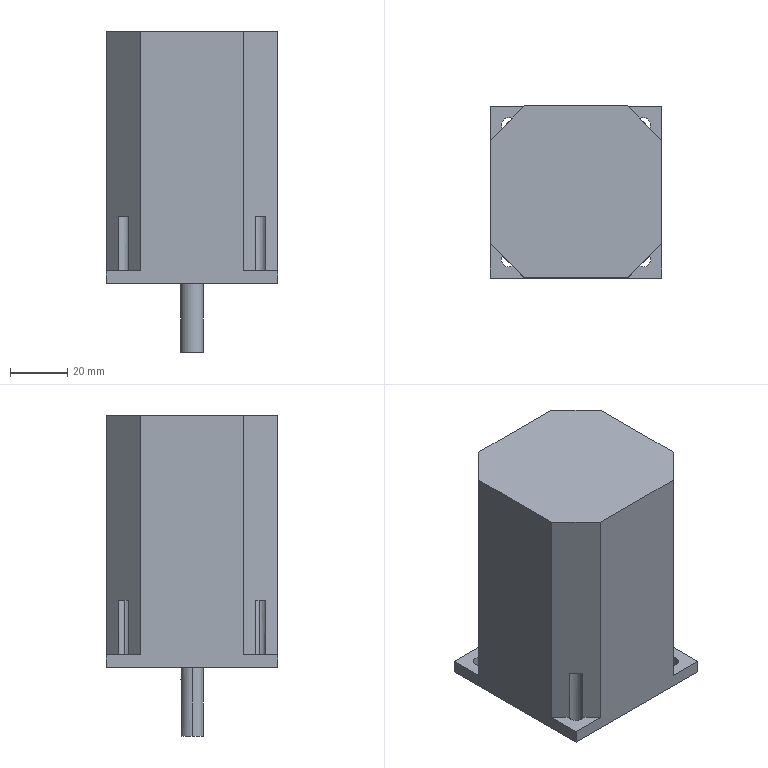Part | 1 solid | 31 faces | box 60 x 60 x 112 mm | volume 292604 mm3 | plane 21 | cylinder 10 | commonest cylinder face diameters 5 x8 8 x2
STEP:
#1=CARTESIAN_POINT('',(-4.,0.,-24.));
#2=VERTEX_POINT('',#1);
#3=CARTESIAN_POINT('',(-1.936,3.5,-24.));
#4=VERTEX_POINT('',#3);
#5=CARTESIAN_POINT('',(0.,0.,-24.));
#6=DIRECTION('',(0.,0.,-1.));
#7=DIRECTION('',(-1.,0.,0.));
#8=AXIS2_PLACEMENT_3D('',#5,#6,#7);
#9=CIRCLE('',#8,4.);
#10=EDGE_CURVE('',#2,#4,#9,.T.);
#11=ORIENTED_EDGE('',*,*,#10,.F.);
#12=CARTESIAN_POINT('',(-4.,0.,0.));
#13=VERTEX_POINT('',#12);
#14=CARTESIAN_POINT('',(-4.,0.,-24.));
#15=DIRECTION('',(0.,0.,1.));
#16=VECTOR('',#15,1000.);
#17=LINE('',#14,#16);
#18=EDGE_CURVE('',#2,#13,#17,.T.);
#19=ORIENTED_EDGE('',*,*,#18,.T.);
#20=CARTESIAN_POINT('',(4.,0.,0.));
#21=VERTEX_POINT('',#20);
#22=CARTESIAN_POINT('',(0.,0.,0.));
#23=DIRECTION('',(0.,0.,-1.));
#24=DIRECTION('',(-1.,0.,0.));
#25=AXIS2_PLACEMENT_3D('',#22,#23,#24);
#26=CIRCLE('',#25,4.);
#27=EDGE_CURVE('',#13,#21,#26,.T.);
#28=ORIENTED_EDGE('',*,*,#27,.T.);
#29=CARTESIAN_POINT('',(4.,0.,-24.));
#30=VERTEX_POINT('',#29);
#31=CARTESIAN_POINT('',(4.,0.,-24.));
#32=DIRECTION('',(0.,0.,1.));
#33=VECTOR('',#32,1000.);
#34=LINE('',#31,#33);
#35=EDGE_CURVE('',#30,#21,#34,.T.);
#36=ORIENTED_EDGE('',*,*,#35,.F.);
#37=CARTESIAN_POINT('',(1.936,3.5,-24.));
#38=VERTEX_POINT('',#37);
#39=CARTESIAN_POINT('',(0.,0.,-24.));
#40=DIRECTION('',(0.,0.,-1.));
#41=DIRECTION('',(-1.,0.,0.));
#42=AXIS2_PLACEMENT_3D('',#39,#40,#41);
#43=CIRCLE('',#42,4.);
#44=EDGE_CURVE('',#38,#30,#43,.T.);
#45=ORIENTED_EDGE('',*,*,#44,.F.);
#46=CARTESIAN_POINT('',(1.936,3.5,-4.));
#47=VERTEX_POINT('',#46);
#48=CARTESIAN_POINT('',(1.936,3.5,-24.));
#49=DIRECTION('',(0.,0.,1.));
#50=VECTOR('',#49,1000.);
#51=LINE('',#48,#50);
#52=EDGE_CURVE('',#38,#47,#51,.T.);
#53=ORIENTED_EDGE('',*,*,#52,.T.);
#54=CARTESIAN_POINT('',(-1.936,3.5,-4.));
#55=VERTEX_POINT('',#54);
#56=CARTESIAN_POINT('',(0.,0.,-4.));
#57=DIRECTION('',(0.,0.,1.));
#58=DIRECTION('',(1.,0.,0.));
#59=AXIS2_PLACEMENT_3D('',#56,#57,#58);
#60=CIRCLE('',#59,4.);
#61=EDGE_CURVE('',#47,#55,#60,.T.);
#62=ORIENTED_EDGE('',*,*,#61,.T.);
#63=CARTESIAN_POINT('',(-1.936,3.5,-24.));
#64=DIRECTION('',(0.,0.,-1.));
#65=VECTOR('',#64,1000.);
#66=LINE('',#63,#65);
#67=EDGE_CURVE('',#55,#4,#66,.T.);
#68=ORIENTED_EDGE('',*,*,#67,.T.);
#69=EDGE_LOOP('',(#11,#19,#28,#36,#45,#53,#62,#68));
#70=FACE_OUTER_BOUND('',#69,.T.);
#71=CARTESIAN_POINT('',(0.,0.,-24.));
#72=DIRECTION('',(0.,0.,1.));
#73=DIRECTION('',(1.,0.,0.));
#74=AXIS2_PLACEMENT_3D('',#71,#72,#73);
#75=CYLINDRICAL_SURFACE('',#74,4.);
#76=ADVANCED_FACE('',(#70),#75,.T.);
#77=CARTESIAN_POINT('',(-21.07,-23.57,23.5));
#78=VERTEX_POINT('',#77);
#79=CARTESIAN_POINT('',(-22.285,-25.715,23.5));
#80=VERTEX_POINT('',#79);
#81=CARTESIAN_POINT('',(-23.57,-23.57,23.5));
#82=DIRECTION('',(0.,0.,-1.));
#83=DIRECTION('',(-1.,0.,0.));
#84=AXIS2_PLACEMENT_3D('',#81,#82,#83);
#85=CIRCLE('',#84,2.5);
#86=EDGE_CURVE('',#78,#80,#85,.T.);
#87=ORIENTED_EDGE('',*,*,#86,.F.);
#88=CARTESIAN_POINT('',(-21.07,-23.57,0.));
#89=VERTEX_POINT('',#88);
#90=CARTESIAN_POINT('',(-21.07,-23.57,23.5));
#91=DIRECTION('',(0.,0.,-1.));
#92=VECTOR('',#91,1000.);
#93=LINE('',#90,#92);
#94=EDGE_CURVE('',#78,#89,#93,.T.);
#95=ORIENTED_EDGE('',*,*,#94,.T.);
#96=CARTESIAN_POINT('',(-26.07,-23.57,0.));
#97=VERTEX_POINT('',#96);
#98=CARTESIAN_POINT('',(-23.57,-23.57,0.));
#99=DIRECTION('',(0.,0.,-1.));
#100=DIRECTION('',(-1.,0.,0.));
#101=AXIS2_PLACEMENT_3D('',#98,#99,#100);
#102=CIRCLE('',#101,2.5);
#103=EDGE_CURVE('',#89,#97,#102,.T.);
#104=ORIENTED_EDGE('',*,*,#103,.T.);
#105=CARTESIAN_POINT('',(-26.07,-23.57,4.5));
#106=VERTEX_POINT('',#105);
#107=CARTESIAN_POINT('',(-26.07,-23.57,23.5));
#108=DIRECTION('',(0.,0.,-1.));
#109=VECTOR('',#108,1000.);
#110=LINE('',#107,#109);
#111=EDGE_CURVE('',#106,#97,#110,.T.);
#112=ORIENTED_EDGE('',*,*,#111,.F.);
#113=CARTESIAN_POINT('',(-22.285,-25.715,4.5));
#114=VERTEX_POINT('',#113);
#115=CARTESIAN_POINT('',(-23.57,-23.57,4.5));
#116=DIRECTION('',(0.,0.,-1.));
#117=DIRECTION('',(-1.,0.,0.));
#118=AXIS2_PLACEMENT_3D('',#115,#116,#117);
#119=CIRCLE('',#118,2.5);
#120=EDGE_CURVE('',#114,#106,#119,.T.);
#121=ORIENTED_EDGE('',*,*,#120,.F.);
#122=CARTESIAN_POINT('',(-22.285,-25.715,23.5));
#123=DIRECTION('',(0.,0.,-1.));
#124=VECTOR('',#123,1000.);
#125=LINE('',#122,#124);
#126=EDGE_CURVE('',#80,#114,#125,.T.);
#127=ORIENTED_EDGE('',*,*,#126,.F.);
#128=EDGE_LOOP('',(#87,#95,#104,#112,#121,#127));
#129=FACE_OUTER_BOUND('',#128,.T.);
#130=CARTESIAN_POINT('',(-23.57,-23.57,23.5));
#131=DIRECTION('',(0.,0.,-1.));
#132=DIRECTION('',(-1.,0.,0.));
#133=AXIS2_PLACEMENT_3D('',#130,#131,#132);
#134=CYLINDRICAL_SURFACE('',#133,2.5);
#135=ADVANCED_FACE('',(#129),#134,.F.);
#136=CARTESIAN_POINT('',(22.285,-25.715,4.5));
#137=VERTEX_POINT('',#136);
#138=CARTESIAN_POINT('',(26.07,-23.57,4.5));
#139=VERTEX_POINT('',#138);
#140=CARTESIAN_POINT('',(23.57,-23.57,4.5));
#141=DIRECTION('',(0.,0.,1.));
#142=DIRECTION('',(1.,0.,0.));
#143=AXIS2_PLACEMENT_3D('',#140,#141,#142);
#144=CIRCLE('',#143,2.5);
#145=EDGE_CURVE('',#137,#139,#144,.T.);
#146=ORIENTED_EDGE('',*,*,#145,.T.);
#147=CARTESIAN_POINT('',(26.07,-23.57,0.));
#148=VERTEX_POINT('',#147);
#149=CARTESIAN_POINT('',(26.07,-23.57,23.5));
#150=DIRECTION('',(0.,0.,-1.));
#151=VECTOR('',#150,1000.);
#152=LINE('',#149,#151);
#153=EDGE_CURVE('',#139,#148,#152,.T.);
#154=ORIENTED_EDGE('',*,*,#153,.T.);
#155=CARTESIAN_POINT('',(21.07,-23.57,0.));
#156=VERTEX_POINT('',#155);
#157=CARTESIAN_POINT('',(23.57,-23.57,0.));
#158=DIRECTION('',(0.,0.,-1.));
#159=DIRECTION('',(-1.,0.,0.));
#160=AXIS2_PLACEMENT_3D('',#157,#158,#159);
#161=CIRCLE('',#160,2.5);
#162=EDGE_CURVE('',#148,#156,#161,.T.);
#163=ORIENTED_EDGE('',*,*,#162,.T.);
#164=CARTESIAN_POINT('',(21.07,-23.57,23.5));
#165=VERTEX_POINT('',#164);
#166=CARTESIAN_POINT('',(21.07,-23.57,23.5));
#167=DIRECTION('',(0.,0.,-1.));
#168=VECTOR('',#167,1000.);
#169=LINE('',#166,#168);
#170=EDGE_CURVE('',#165,#156,#169,.T.);
#171=ORIENTED_EDGE('',*,*,#170,.F.);
#172=CARTESIAN_POINT('',(22.285,-25.715,23.5));
#173=VERTEX_POINT('',#172);
#174=CARTESIAN_POINT('',(23.57,-23.57,23.5));
#175=DIRECTION('',(0.,0.,-1.));
#176=DIRECTION('',(-1.,0.,0.));
#177=AXIS2_PLACEMENT_3D('',#174,#175,#176);
#178=CIRCLE('',#177,2.5);
#179=EDGE_CURVE('',#173,#165,#178,.T.);
#180=ORIENTED_EDGE('',*,*,#179,.F.);
#181=CARTESIAN_POINT('',(22.285,-25.715,23.5));
#182=DIRECTION('',(0.,0.,1.));
#183=VECTOR('',#182,1000.);
#184=LINE('',#181,#183);
#185=EDGE_CURVE('',#137,#173,#184,.T.);
#186=ORIENTED_EDGE('',*,*,#185,.F.);
#187=EDGE_LOOP('',(#146,#154,#163,#171,#180,#186));
#188=FACE_OUTER_BOUND('',#187,.T.);
#189=CARTESIAN_POINT('',(23.57,-23.57,23.5));
#190=DIRECTION('',(0.,0.,-1.));
#191=DIRECTION('',(-1.,0.,0.));
#192=AXIS2_PLACEMENT_3D('',#189,#190,#191);
#193=CYLINDRICAL_SURFACE('',#192,2.5);
#194=ADVANCED_FACE('',(#188),#193,.F.);
#195=CARTESIAN_POINT('',(-21.07,23.57,23.5));
#196=VERTEX_POINT('',#195);
#197=CARTESIAN_POINT('',(-25.715,22.285,23.5));
#198=VERTEX_POINT('',#197);
#199=CARTESIAN_POINT('',(-23.57,23.57,23.5));
#200=DIRECTION('',(0.,0.,-1.));
#201=DIRECTION('',(-1.,0.,0.));
#202=AXIS2_PLACEMENT_3D('',#199,#200,#201);
#203=CIRCLE('',#202,2.5);
#204=EDGE_CURVE('',#196,#198,#203,.T.);
#205=ORIENTED_EDGE('',*,*,#204,.F.);
#206=CARTESIAN_POINT('',(-21.07,23.57,0.));
#207=VERTEX_POINT('',#206);
#208=CARTESIAN_POINT('',(-21.07,23.57,23.5));
#209=DIRECTION('',(0.,0.,-1.));
#210=VECTOR('',#209,1000.);
#211=LINE('',#208,#210);
#212=EDGE_CURVE('',#196,#207,#211,.T.);
#213=ORIENTED_EDGE('',*,*,#212,.T.);
#214=CARTESIAN_POINT('',(-26.07,23.57,0.));
#215=VERTEX_POINT('',#214);
#216=CARTESIAN_POINT('',(-23.57,23.57,0.));
#217=DIRECTION('',(0.,0.,-1.));
#218=DIRECTION('',(-1.,0.,0.));
#219=AXIS2_PLACEMENT_3D('',#216,#217,#218);
#220=CIRCLE('',#219,2.5);
#221=EDGE_CURVE('',#207,#215,#220,.T.);
#222=ORIENTED_EDGE('',*,*,#221,.T.);
#223=CARTESIAN_POINT('',(-26.07,23.57,4.5));
#224=VERTEX_POINT('',#223);
#225=CARTESIAN_POINT('',(-26.07,23.57,23.5));
#226=DIRECTION('',(0.,0.,-1.));
#227=VECTOR('',#226,1000.);
#228=LINE('',#225,#227);
#229=EDGE_CURVE('',#224,#215,#228,.T.);
#230=ORIENTED_EDGE('',*,*,#229,.F.);
#231=CARTESIAN_POINT('',(-25.715,22.285,4.5));
#232=VERTEX_POINT('',#231);
#233=CARTESIAN_POINT('',(-23.57,23.57,4.5));
#234=DIRECTION('',(0.,0.,1.));
#235=DIRECTION('',(1.,0.,0.));
#236=AXIS2_PLACEMENT_3D('',#233,#234,#235);
#237=CIRCLE('',#236,2.5);
#238=EDGE_CURVE('',#224,#232,#237,.T.);
#239=ORIENTED_EDGE('',*,*,#238,.T.);
#240=CARTESIAN_POINT('',(-25.715,22.285,23.5));
#241=DIRECTION('',(0.,0.,-1.));
#242=VECTOR('',#241,1000.);
#243=LINE('',#240,#242);
#244=EDGE_CURVE('',#198,#232,#243,.T.);
#245=ORIENTED_EDGE('',*,*,#244,.F.);
#246=EDGE_LOOP('',(#205,#213,#222,#230,#239,#245));
#247=FACE_OUTER_BOUND('',#246,.T.);
#248=CARTESIAN_POINT('',(-23.57,23.57,23.5));
#249=DIRECTION('',(0.,0.,-1.));
#250=DIRECTION('',(-1.,0.,0.));
#251=AXIS2_PLACEMENT_3D('',#248,#249,#250);
#252=CYLINDRICAL_SURFACE('',#251,2.5);
#253=ADVANCED_FACE('',(#247),#252,.F.);
#254=CARTESIAN_POINT('',(26.07,23.57,4.5));
#255=VERTEX_POINT('',#254);
#256=CARTESIAN_POINT('',(25.715,22.285,4.5));
#257=VERTEX_POINT('',#256);
#258=CARTESIAN_POINT('',(23.57,23.57,4.5));
#259=DIRECTION('',(0.,0.,-1.));
#260=DIRECTION('',(-1.,0.,0.));
#261=AXIS2_PLACEMENT_3D('',#258,#259,#260);
#262=CIRCLE('',#261,2.5);
#263=EDGE_CURVE('',#255,#257,#262,.T.);
#264=ORIENTED_EDGE('',*,*,#263,.F.);
#265=CARTESIAN_POINT('',(26.07,23.57,0.));
#266=VERTEX_POINT('',#265);
#267=CARTESIAN_POINT('',(26.07,23.57,23.5));
#268=DIRECTION('',(0.,0.,-1.));
#269=VECTOR('',#268,1000.);
#270=LINE('',#267,#269);
#271=EDGE_CURVE('',#255,#266,#270,.T.);
#272=ORIENTED_EDGE('',*,*,#271,.T.);
#273=CARTESIAN_POINT('',(21.07,23.57,0.));
#274=VERTEX_POINT('',#273);
#275=CARTESIAN_POINT('',(23.57,23.57,0.));
#276=DIRECTION('',(0.,0.,-1.));
#277=DIRECTION('',(-1.,0.,0.));
#278=AXIS2_PLACEMENT_3D('',#275,#276,#277);
#279=CIRCLE('',#278,2.5);
#280=EDGE_CURVE('',#266,#274,#279,.T.);
#281=ORIENTED_EDGE('',*,*,#280,.T.);
#282=CARTESIAN_POINT('',(21.07,23.57,23.5));
#283=VERTEX_POINT('',#282);
#284=CARTESIAN_POINT('',(21.07,23.57,23.5));
#285=DIRECTION('',(0.,0.,-1.));
#286=VECTOR('',#285,1000.);
#287=LINE('',#284,#286);
#288=EDGE_CURVE('',#283,#274,#287,.T.);
#289=ORIENTED_EDGE('',*,*,#288,.F.);
#290=CARTESIAN_POINT('',(25.715,22.285,23.5));
#291=VERTEX_POINT('',#290);
#292=CARTESIAN_POINT('',(23.57,23.57,23.5));
#293=DIRECTION('',(0.,0.,-1.));
#294=DIRECTION('',(-1.,0.,0.));
#295=AXIS2_PLACEMENT_3D('',#292,#293,#294);
#296=CIRCLE('',#295,2.5);
#297=EDGE_CURVE('',#291,#283,#296,.T.);
#298=ORIENTED_EDGE('',*,*,#297,.F.);
#299=CARTESIAN_POINT('',(25.715,22.285,23.5));
#300=DIRECTION('',(0.,0.,1.));
#301=VECTOR('',#300,1000.);
#302=LINE('',#299,#301);
#303=EDGE_CURVE('',#257,#291,#302,.T.);
#304=ORIENTED_EDGE('',*,*,#303,.F.);
#305=EDGE_LOOP('',(#264,#272,#281,#289,#298,#304));
#306=FACE_OUTER_BOUND('',#305,.T.);
#307=CARTESIAN_POINT('',(23.57,23.57,23.5));
#308=DIRECTION('',(0.,0.,-1.));
#309=DIRECTION('',(-1.,0.,0.));
#310=AXIS2_PLACEMENT_3D('',#307,#308,#309);
#311=CYLINDRICAL_SURFACE('',#310,2.5);
#312=ADVANCED_FACE('',(#306),#311,.F.);
#313=CARTESIAN_POINT('',(30.,-30.,0.));
#314=VERTEX_POINT('',#313);
#315=CARTESIAN_POINT('',(30.,30.,0.));
#316=VERTEX_POINT('',#315);
#317=CARTESIAN_POINT('',(30.,-30.,0.));
#318=DIRECTION('',(0.,1.,0.));
#319=VECTOR('',#318,1000.);
#320=LINE('',#317,#319);
#321=EDGE_CURVE('',#314,#316,#320,.T.);
#322=ORIENTED_EDGE('',*,*,#321,.F.);
#323=CARTESIAN_POINT('',(-30.,-30.,0.));
#324=VERTEX_POINT('',#323);
#325=CARTESIAN_POINT('',(-30.,-30.,0.));
#326=DIRECTION('',(1.,0.,0.));
#327=VECTOR('',#326,1000.);
#328=LINE('',#325,#327);
#329=EDGE_CURVE('',#324,#314,#328,.T.);
#330=ORIENTED_EDGE('',*,*,#329,.F.);
#331=CARTESIAN_POINT('',(-30.,30.,0.));
#332=VERTEX_POINT('',#331);
#333=CARTESIAN_POINT('',(-30.,-30.,0.));
#334=DIRECTION('',(0.,-1.,0.));
#335=VECTOR('',#334,1000.);
#336=LINE('',#333,#335);
#337=EDGE_CURVE('',#332,#324,#336,.T.);
#338=ORIENTED_EDGE('',*,*,#337,.F.);
#339=CARTESIAN_POINT('',(-30.,30.,0.));
#340=DIRECTION('',(-1.,0.,0.));
#341=VECTOR('',#340,1000.);
#342=LINE('',#339,#341);
#343=EDGE_CURVE('',#316,#332,#342,.T.);
#344=ORIENTED_EDGE('',*,*,#343,.F.);
#345=EDGE_LOOP('',(#322,#330,#338,#344));
#346=FACE_OUTER_BOUND('',#345,.T.);
#347=CARTESIAN_POINT('',(23.57,23.57,0.));
#348=DIRECTION('',(0.,0.,-1.));
#349=DIRECTION('',(-1.,0.,0.));
#350=AXIS2_PLACEMENT_3D('',#347,#348,#349);
#351=CIRCLE('',#350,2.5);
#352=EDGE_CURVE('',#274,#266,#351,.T.);
#353=ORIENTED_EDGE('',*,*,#352,.F.);
#354=ORIENTED_EDGE('',*,*,#280,.F.);
#355=EDGE_LOOP('',(#353,#354));
#356=FACE_BOUND('',#355,.T.);
#357=CARTESIAN_POINT('',(-23.57,23.57,0.));
#358=DIRECTION('',(0.,0.,-1.));
#359=DIRECTION('',(-1.,0.,0.));
#360=AXIS2_PLACEMENT_3D('',#357,#358,#359);
#361=CIRCLE('',#360,2.5);
#362=EDGE_CURVE('',#215,#207,#361,.T.);
#363=ORIENTED_EDGE('',*,*,#362,.F.);
#364=ORIENTED_EDGE('',*,*,#221,.F.);
#365=EDGE_LOOP('',(#363,#364));
#366=FACE_BOUND('',#365,.T.);
#367=CARTESIAN_POINT('',(23.57,-23.57,0.));
#368=DIRECTION('',(0.,0.,-1.));
#369=DIRECTION('',(-1.,0.,0.));
#370=AXIS2_PLACEMENT_3D('',#367,#368,#369);
#371=CIRCLE('',#370,2.5);
#372=EDGE_CURVE('',#156,#148,#371,.T.);
#373=ORIENTED_EDGE('',*,*,#372,.F.);
#374=ORIENTED_EDGE('',*,*,#162,.F.);
#375=EDGE_LOOP('',(#373,#374));
#376=FACE_BOUND('',#375,.T.);
#377=CARTESIAN_POINT('',(-23.57,-23.57,0.));
#378=DIRECTION('',(0.,0.,-1.));
#379=DIRECTION('',(-1.,0.,0.));
#380=AXIS2_PLACEMENT_3D('',#377,#378,#379);
#381=CIRCLE('',#380,2.5);
#382=EDGE_CURVE('',#97,#89,#381,.T.);
#383=ORIENTED_EDGE('',*,*,#382,.F.);
#384=ORIENTED_EDGE('',*,*,#103,.F.);
#385=EDGE_LOOP('',(#383,#384));
#386=FACE_BOUND('',#385,.T.);
#387=CARTESIAN_POINT('',(0.,0.,0.));
#388=DIRECTION('',(0.,0.,-1.));
#389=DIRECTION('',(-1.,0.,0.));
#390=AXIS2_PLACEMENT_3D('',#387,#388,#389);
#391=CIRCLE('',#390,4.);
#392=EDGE_CURVE('',#21,#13,#391,.T.);
#393=ORIENTED_EDGE('',*,*,#392,.F.);
#394=ORIENTED_EDGE('',*,*,#27,.F.);
#395=EDGE_LOOP('',(#393,#394));
#396=FACE_BOUND('',#395,.T.);
#397=CARTESIAN_POINT('',(0.,0.,0.));
#398=DIRECTION('',(0.,0.,-1.));
#399=DIRECTION('',(-1.,0.,0.));
#400=AXIS2_PLACEMENT_3D('',#397,#398,#399);
#401=PLANE('',#400);
#402=ADVANCED_FACE('',(#346,#356,#366,#376,#386,#396),#401,.T.);
#403=CARTESIAN_POINT('',(30.,18.,4.5));
#404=VERTEX_POINT('',#403);
#405=CARTESIAN_POINT('',(30.,30.,4.5));
#406=VERTEX_POINT('',#405);
#407=CARTESIAN_POINT('',(30.,30.,4.5));
#408=DIRECTION('',(0.,1.,0.));
#409=VECTOR('',#408,1000.);
#410=LINE('',#407,#409);
#411=EDGE_CURVE('',#404,#406,#410,.T.);
#412=ORIENTED_EDGE('',*,*,#411,.F.);
#413=CARTESIAN_POINT('',(30.,18.,88.));
#414=VERTEX_POINT('',#413);
#415=CARTESIAN_POINT('',(30.,18.,4.5));
#416=DIRECTION('',(0.,0.,1.));
#417=VECTOR('',#416,1000.);
#418=LINE('',#415,#417);
#419=EDGE_CURVE('',#404,#414,#418,.T.);
#420=ORIENTED_EDGE('',*,*,#419,.T.);
#421=CARTESIAN_POINT('',(30.,-18.,88.));
#422=VERTEX_POINT('',#421);
#423=CARTESIAN_POINT('',(30.,-30.,88.));
#424=DIRECTION('',(0.,1.,0.));
#425=VECTOR('',#424,1000.);
#426=LINE('',#423,#425);
#427=EDGE_CURVE('',#422,#414,#426,.T.);
#428=ORIENTED_EDGE('',*,*,#427,.F.);
#429=CARTESIAN_POINT('',(30.,-18.,4.5));
#430=VERTEX_POINT('',#429);
#431=CARTESIAN_POINT('',(30.,-18.,4.5));
#432=DIRECTION('',(0.,0.,1.));
#433=VECTOR('',#432,1000.);
#434=LINE('',#431,#433);
#435=EDGE_CURVE('',#430,#422,#434,.T.);
#436=ORIENTED_EDGE('',*,*,#435,.F.);
#437=CARTESIAN_POINT('',(30.,-30.,4.5));
#438=VERTEX_POINT('',#437);
#439=CARTESIAN_POINT('',(30.,-30.,4.5));
#440=DIRECTION('',(0.,1.,0.));
#441=VECTOR('',#440,1000.);
#442=LINE('',#439,#441);
#443=EDGE_CURVE('',#438,#430,#442,.T.);
#444=ORIENTED_EDGE('',*,*,#443,.F.);
#445=CARTESIAN_POINT('',(30.,-30.,88.));
#446=DIRECTION('',(0.,0.,-1.));
#447=VECTOR('',#446,1000.);
#448=LINE('',#445,#447);
#449=EDGE_CURVE('',#438,#314,#448,.T.);
#450=ORIENTED_EDGE('',*,*,#449,.T.);
#451=ORIENTED_EDGE('',*,*,#321,.T.);
#452=CARTESIAN_POINT('',(30.,30.,88.));
#453=DIRECTION('',(0.,0.,-1.));
#454=VECTOR('',#453,1000.);
#455=LINE('',#452,#454);
#456=EDGE_CURVE('',#406,#316,#455,.T.);
#457=ORIENTED_EDGE('',*,*,#456,.F.);
#458=EDGE_LOOP('',(#412,#420,#428,#436,#444,#450,#451,#457));
#459=FACE_OUTER_BOUND('',#458,.T.);
#460=CARTESIAN_POINT('',(30.,-30.,88.));
#461=DIRECTION('',(-1.,0.,0.));
#462=DIRECTION('',(0.,0.,1.));
#463=AXIS2_PLACEMENT_3D('',#460,#461,#462);
#464=PLANE('',#463);
#465=ADVANCED_FACE('',(#459),#464,.F.);
#466=CARTESIAN_POINT('',(18.,30.,88.));
#467=VERTEX_POINT('',#466);
#468=CARTESIAN_POINT('',(-18.,30.,88.));
#469=VERTEX_POINT('',#468);
#470=CARTESIAN_POINT('',(-30.,30.,88.));
#471=DIRECTION('',(-1.,0.,0.));
#472=VECTOR('',#471,1000.);
#473=LINE('',#470,#472);
#474=EDGE_CURVE('',#467,#469,#473,.T.);
#475=ORIENTED_EDGE('',*,*,#474,.F.);
#476=CARTESIAN_POINT('',(18.,30.,4.5));
#477=VERTEX_POINT('',#476);
#478=CARTESIAN_POINT('',(18.,30.,4.5));
#479=DIRECTION('',(0.,0.,1.));
#480=VECTOR('',#479,1000.);
#481=LINE('',#478,#480);
#482=EDGE_CURVE('',#477,#467,#481,.T.);
#483=ORIENTED_EDGE('',*,*,#482,.F.);
#484=CARTESIAN_POINT('',(18.,30.,4.5));
#485=DIRECTION('',(-1.,0.,0.));
#486=VECTOR('',#485,1000.);
#487=LINE('',#484,#486);
#488=EDGE_CURVE('',#406,#477,#487,.T.);
#489=ORIENTED_EDGE('',*,*,#488,.F.);
#490=ORIENTED_EDGE('',*,*,#456,.T.);
#491=ORIENTED_EDGE('',*,*,#343,.T.);
#492=CARTESIAN_POINT('',(-30.,30.,4.5));
#493=VERTEX_POINT('',#492);
#494=CARTESIAN_POINT('',(-30.,30.,88.));
#495=DIRECTION('',(0.,0.,-1.));
#496=VECTOR('',#495,1000.);
#497=LINE('',#494,#496);
#498=EDGE_CURVE('',#493,#332,#497,.T.);
#499=ORIENTED_EDGE('',*,*,#498,.F.);
#500=CARTESIAN_POINT('',(-18.,30.,4.5));
#501=VERTEX_POINT('',#500);
#502=CARTESIAN_POINT('',(-18.,30.,4.5));
#503=DIRECTION('',(-1.,0.,0.));
#504=VECTOR('',#503,1000.);
#505=LINE('',#502,#504);
#506=EDGE_CURVE('',#501,#493,#505,.T.);
#507=ORIENTED_EDGE('',*,*,#506,.F.);
#508=CARTESIAN_POINT('',(-18.,30.,4.5));
#509=DIRECTION('',(0.,0.,1.));
#510=VECTOR('',#509,1000.);
#511=LINE('',#508,#510);
#512=EDGE_CURVE('',#501,#469,#511,.T.);
#513=ORIENTED_EDGE('',*,*,#512,.T.);
#514=EDGE_LOOP('',(#475,#483,#489,#490,#491,#499,#507,#513));
#515=FACE_OUTER_BOUND('',#514,.T.);
#516=CARTESIAN_POINT('',(-30.,30.,88.));
#517=DIRECTION('',(0.,-1.,0.));
#518=DIRECTION('',(0.,0.,-1.));
#519=AXIS2_PLACEMENT_3D('',#516,#517,#518);
#520=PLANE('',#519);
#521=ADVANCED_FACE('',(#515),#520,.F.);
#522=CARTESIAN_POINT('',(-30.,-18.,4.5));
#523=VERTEX_POINT('',#522);
#524=CARTESIAN_POINT('',(-30.,-30.,4.5));
#525=VERTEX_POINT('',#524);
#526=CARTESIAN_POINT('',(-30.,-30.,4.5));
#527=DIRECTION('',(0.,-1.,0.));
#528=VECTOR('',#527,1000.);
#529=LINE('',#526,#528);
#530=EDGE_CURVE('',#523,#525,#529,.T.);
#531=ORIENTED_EDGE('',*,*,#530,.F.);
#532=CARTESIAN_POINT('',(-30.,-18.,88.));
#533=VERTEX_POINT('',#532);
#534=CARTESIAN_POINT('',(-30.,-18.,4.5));
#535=DIRECTION('',(0.,0.,1.));
#536=VECTOR('',#535,1000.);
#537=LINE('',#534,#536);
#538=EDGE_CURVE('',#523,#533,#537,.T.);
#539=ORIENTED_EDGE('',*,*,#538,.T.);
#540=CARTESIAN_POINT('',(-30.,18.,88.));
#541=VERTEX_POINT('',#540);
#542=CARTESIAN_POINT('',(-30.,-30.,88.));
#543=DIRECTION('',(0.,-1.,0.));
#544=VECTOR('',#543,1000.);
#545=LINE('',#542,#544);
#546=EDGE_CURVE('',#541,#533,#545,.T.);
#547=ORIENTED_EDGE('',*,*,#546,.F.);
#548=CARTESIAN_POINT('',(-30.,18.,4.5));
#549=VERTEX_POINT('',#548);
#550=CARTESIAN_POINT('',(-30.,18.,4.5));
#551=DIRECTION('',(0.,0.,1.));
#552=VECTOR('',#551,1000.);
#553=LINE('',#550,#552);
#554=EDGE_CURVE('',#549,#541,#553,.T.);
#555=ORIENTED_EDGE('',*,*,#554,.F.);
#556=CARTESIAN_POINT('',(-30.,30.,4.5));
#557=DIRECTION('',(0.,-1.,0.));
#558=VECTOR('',#557,1000.);
#559=LINE('',#556,#558);
#560=EDGE_CURVE('',#493,#549,#559,.T.);
#561=ORIENTED_EDGE('',*,*,#560,.F.);
#562=ORIENTED_EDGE('',*,*,#498,.T.);
#563=ORIENTED_EDGE('',*,*,#337,.T.);
#564=CARTESIAN_POINT('',(-30.,-30.,88.));
#565=DIRECTION('',(0.,0.,-1.));
#566=VECTOR('',#565,1000.);
#567=LINE('',#564,#566);
#568=EDGE_CURVE('',#525,#324,#567,.T.);
#569=ORIENTED_EDGE('',*,*,#568,.F.);
#570=EDGE_LOOP('',(#531,#539,#547,#555,#561,#562,#563,#569));
#571=FACE_OUTER_BOUND('',#570,.T.);
#572=CARTESIAN_POINT('',(-30.,-30.,88.));
#573=DIRECTION('',(1.,0.,0.));
#574=DIRECTION('',(0.,0.,-1.));
#575=AXIS2_PLACEMENT_3D('',#572,#573,#574);
#576=PLANE('',#575);
#577=ADVANCED_FACE('',(#571),#576,.F.);
#578=CARTESIAN_POINT('',(18.,-30.,4.5));
#579=VERTEX_POINT('',#578);
#580=CARTESIAN_POINT('',(18.,-30.,4.5));
#581=DIRECTION('',(1.,0.,0.));
#582=VECTOR('',#581,1000.);
#583=LINE('',#580,#582);
#584=EDGE_CURVE('',#579,#438,#583,.T.);
#585=ORIENTED_EDGE('',*,*,#584,.F.);
#586=CARTESIAN_POINT('',(18.,-30.,88.));
#587=VERTEX_POINT('',#586);
#588=CARTESIAN_POINT('',(18.,-30.,4.5));
#589=DIRECTION('',(0.,0.,1.));
#590=VECTOR('',#589,1000.);
#591=LINE('',#588,#590);
#592=EDGE_CURVE('',#579,#587,#591,.T.);
#593=ORIENTED_EDGE('',*,*,#592,.T.);
#594=CARTESIAN_POINT('',(-18.,-30.,88.));
#595=VERTEX_POINT('',#594);
#596=CARTESIAN_POINT('',(-30.,-30.,88.));
#597=DIRECTION('',(1.,0.,0.));
#598=VECTOR('',#597,1000.);
#599=LINE('',#596,#598);
#600=EDGE_CURVE('',#595,#587,#599,.T.);
#601=ORIENTED_EDGE('',*,*,#600,.F.);
#602=CARTESIAN_POINT('',(-18.,-30.,4.5));
#603=VERTEX_POINT('',#602);
#604=CARTESIAN_POINT('',(-18.,-30.,4.5));
#605=DIRECTION('',(0.,0.,1.));
#606=VECTOR('',#605,1000.);
#607=LINE('',#604,#606);
#608=EDGE_CURVE('',#603,#595,#607,.T.);
#609=ORIENTED_EDGE('',*,*,#608,.F.);
#610=CARTESIAN_POINT('',(-18.,-30.,4.5));
#611=DIRECTION('',(1.,0.,0.));
#612=VECTOR('',#611,1000.);
#613=LINE('',#610,#612);
#614=EDGE_CURVE('',#525,#603,#613,.T.);
#615=ORIENTED_EDGE('',*,*,#614,.F.);
#616=ORIENTED_EDGE('',*,*,#568,.T.);
#617=ORIENTED_EDGE('',*,*,#329,.T.);
#618=ORIENTED_EDGE('',*,*,#449,.F.);
#619=EDGE_LOOP('',(#585,#593,#601,#609,#615,#616,#617,#618));
#620=FACE_OUTER_BOUND('',#619,.T.);
#621=CARTESIAN_POINT('',(-30.,-30.,88.));
#622=DIRECTION('',(0.,1.,0.));
#623=DIRECTION('',(0.,0.,1.));
#624=AXIS2_PLACEMENT_3D('',#621,#622,#623);
#625=PLANE('',#624);
#626=ADVANCED_FACE('',(#620),#625,.F.);
#627=ORIENTED_EDGE('',*,*,#427,.T.);
#628=CARTESIAN_POINT('',(30.,18.,88.));
#629=DIRECTION('',(0.7071,-0.7071,0.));
#630=VECTOR('',#629,1000.);
#631=LINE('',#628,#630);
#632=EDGE_CURVE('',#467,#414,#631,.T.);
#633=ORIENTED_EDGE('',*,*,#632,.F.);
#634=ORIENTED_EDGE('',*,*,#474,.T.);
#635=CARTESIAN_POINT('',(-30.,18.,88.));
#636=DIRECTION('',(0.7071,0.7071,0.));
#637=VECTOR('',#636,1000.);
#638=LINE('',#635,#637);
#639=EDGE_CURVE('',#541,#469,#638,.T.);
#640=ORIENTED_EDGE('',*,*,#639,.F.);
#641=ORIENTED_EDGE('',*,*,#546,.T.);
#642=CARTESIAN_POINT('',(-30.,-18.,88.));
#643=DIRECTION('',(-0.7071,0.7071,0.));
#644=VECTOR('',#643,1000.);
#645=LINE('',#642,#644);
#646=EDGE_CURVE('',#595,#533,#645,.T.);
#647=ORIENTED_EDGE('',*,*,#646,.F.);
#648=ORIENTED_EDGE('',*,*,#600,.T.);
#649=CARTESIAN_POINT('',(30.,-18.,88.));
#650=DIRECTION('',(-0.7071,-0.7071,0.));
#651=VECTOR('',#650,1000.);
#652=LINE('',#649,#651);
#653=EDGE_CURVE('',#422,#587,#652,.T.);
#654=ORIENTED_EDGE('',*,*,#653,.F.);
#655=EDGE_LOOP('',(#627,#633,#634,#640,#641,#647,#648,#654));
#656=FACE_OUTER_BOUND('',#655,.T.);
#657=CARTESIAN_POINT('',(0.,0.,88.));
#658=DIRECTION('',(0.,0.,-1.));
#659=DIRECTION('',(-1.,0.,0.));
#660=AXIS2_PLACEMENT_3D('',#657,#658,#659);
#661=PLANE('',#660);
#662=ADVANCED_FACE('',(#656),#661,.F.);
#663=CARTESIAN_POINT('',(-22.285,25.715,23.5));
#664=VERTEX_POINT('',#663);
#665=CARTESIAN_POINT('',(-30.,18.,23.5));
#666=DIRECTION('',(0.7071,0.7071,0.));
#667=VECTOR('',#666,1000.);
#668=LINE('',#665,#667);
#669=EDGE_CURVE('',#198,#664,#668,.T.);
#670=ORIENTED_EDGE('',*,*,#669,.F.);
#671=ORIENTED_EDGE('',*,*,#244,.T.);
#672=CARTESIAN_POINT('',(-30.,18.,4.5));
#673=DIRECTION('',(0.7071,0.7071,0.));
#674=VECTOR('',#673,1000.);
#675=LINE('',#672,#674);
#676=EDGE_CURVE('',#549,#232,#675,.T.);
#677=ORIENTED_EDGE('',*,*,#676,.F.);
#678=ORIENTED_EDGE('',*,*,#554,.T.);
#679=ORIENTED_EDGE('',*,*,#639,.T.);
#680=ORIENTED_EDGE('',*,*,#512,.F.);
#681=CARTESIAN_POINT('',(-22.285,25.715,4.5));
#682=VERTEX_POINT('',#681);
#683=CARTESIAN_POINT('',(-30.,18.,4.5));
#684=DIRECTION('',(0.7071,0.7071,0.));
#685=VECTOR('',#684,1000.);
#686=LINE('',#683,#685);
#687=EDGE_CURVE('',#682,#501,#686,.T.);
#688=ORIENTED_EDGE('',*,*,#687,.F.);
#689=CARTESIAN_POINT('',(-22.285,25.715,23.5));
#690=DIRECTION('',(0.,0.,1.));
#691=VECTOR('',#690,1000.);
#692=LINE('',#689,#691);
#693=EDGE_CURVE('',#682,#664,#692,.T.);
#694=ORIENTED_EDGE('',*,*,#693,.T.);
#695=EDGE_LOOP('',(#670,#671,#677,#678,#679,#680,#688,#694));
#696=FACE_OUTER_BOUND('',#695,.T.);
#697=CARTESIAN_POINT('',(-30.,18.,4.5));
#698=DIRECTION('',(0.7071,-0.7071,0.));
#699=DIRECTION('',(0.7071,0.7071,0.));
#700=AXIS2_PLACEMENT_3D('',#697,#698,#699);
#701=PLANE('',#700);
#702=ADVANCED_FACE('',(#696),#701,.F.);
#703=CARTESIAN_POINT('',(-23.57,23.57,4.5));
#704=DIRECTION('',(0.,0.,1.));
#705=DIRECTION('',(1.,0.,0.));
#706=AXIS2_PLACEMENT_3D('',#703,#704,#705);
#707=CIRCLE('',#706,2.5);
#708=EDGE_CURVE('',#682,#224,#707,.T.);
#709=ORIENTED_EDGE('',*,*,#708,.F.);
#710=ORIENTED_EDGE('',*,*,#687,.T.);
#711=ORIENTED_EDGE('',*,*,#506,.T.);
#712=ORIENTED_EDGE('',*,*,#560,.T.);
#713=ORIENTED_EDGE('',*,*,#676,.T.);
#714=ORIENTED_EDGE('',*,*,#238,.F.);
#715=EDGE_LOOP('',(#709,#710,#711,#712,#713,#714));
#716=FACE_OUTER_BOUND('',#715,.T.);
#717=CARTESIAN_POINT('',(0.,0.,4.5));
#718=DIRECTION('',(0.,0.,1.));
#719=DIRECTION('',(1.,0.,0.));
#720=AXIS2_PLACEMENT_3D('',#717,#718,#719);
#721=PLANE('',#720);
#722=ADVANCED_FACE('',(#716),#721,.T.);
#723=CARTESIAN_POINT('',(-25.715,-22.285,23.5));
#724=VERTEX_POINT('',#723);
#725=CARTESIAN_POINT('',(-30.,-18.,23.5));
#726=DIRECTION('',(-0.7071,0.7071,0.));
#727=VECTOR('',#726,1000.);
#728=LINE('',#725,#727);
#729=EDGE_CURVE('',#80,#724,#728,.T.);
#730=ORIENTED_EDGE('',*,*,#729,.F.);
#731=ORIENTED_EDGE('',*,*,#126,.T.);
#732=CARTESIAN_POINT('',(-30.,-18.,4.5));
#733=DIRECTION('',(-0.7071,0.7071,0.));
#734=VECTOR('',#733,1000.);
#735=LINE('',#732,#734);
#736=EDGE_CURVE('',#603,#114,#735,.T.);
#737=ORIENTED_EDGE('',*,*,#736,.F.);
#738=ORIENTED_EDGE('',*,*,#608,.T.);
#739=ORIENTED_EDGE('',*,*,#646,.T.);
#740=ORIENTED_EDGE('',*,*,#538,.F.);
#741=CARTESIAN_POINT('',(-25.715,-22.285,4.5));
#742=VERTEX_POINT('',#741);
#743=CARTESIAN_POINT('',(-30.,-18.,4.5));
#744=DIRECTION('',(-0.7071,0.7071,0.));
#745=VECTOR('',#744,1000.);
#746=LINE('',#743,#745);
#747=EDGE_CURVE('',#742,#523,#746,.T.);
#748=ORIENTED_EDGE('',*,*,#747,.F.);
#749=CARTESIAN_POINT('',(-25.715,-22.285,23.5));
#750=DIRECTION('',(0.,0.,1.));
#751=VECTOR('',#750,1000.);
#752=LINE('',#749,#751);
#753=EDGE_CURVE('',#742,#724,#752,.T.);
#754=ORIENTED_EDGE('',*,*,#753,.T.);
#755=EDGE_LOOP('',(#730,#731,#737,#738,#739,#740,#748,#754));
#756=FACE_OUTER_BOUND('',#755,.T.);
#757=CARTESIAN_POINT('',(-30.,-18.,4.5));
#758=DIRECTION('',(0.7071,0.7071,0.));
#759=DIRECTION('',(-0.7071,0.7071,0.));
#760=AXIS2_PLACEMENT_3D('',#757,#758,#759);
#761=PLANE('',#760);
#762=ADVANCED_FACE('',(#756),#761,.F.);
#763=ORIENTED_EDGE('',*,*,#736,.T.);
#764=ORIENTED_EDGE('',*,*,#120,.T.);
#765=CARTESIAN_POINT('',(-23.57,-23.57,4.5));
#766=DIRECTION('',(0.,0.,-1.));
#767=DIRECTION('',(-1.,0.,0.));
#768=AXIS2_PLACEMENT_3D('',#765,#766,#767);
#769=CIRCLE('',#768,2.5);
#770=EDGE_CURVE('',#106,#742,#769,.T.);
#771=ORIENTED_EDGE('',*,*,#770,.T.);
#772=ORIENTED_EDGE('',*,*,#747,.T.);
#773=ORIENTED_EDGE('',*,*,#530,.T.);
#774=ORIENTED_EDGE('',*,*,#614,.T.);
#775=EDGE_LOOP('',(#763,#764,#771,#772,#773,#774));
#776=FACE_OUTER_BOUND('',#775,.T.);
#777=CARTESIAN_POINT('',(0.,0.,4.5));
#778=DIRECTION('',(0.,0.,-1.));
#779=DIRECTION('',(-1.,0.,0.));
#780=AXIS2_PLACEMENT_3D('',#777,#778,#779);
#781=PLANE('',#780);
#782=ADVANCED_FACE('',(#776),#781,.F.);
#783=CARTESIAN_POINT('',(25.715,-22.285,23.5));
#784=VERTEX_POINT('',#783);
#785=CARTESIAN_POINT('',(30.,-18.,23.5));
#786=DIRECTION('',(-0.7071,-0.7071,0.));
#787=VECTOR('',#786,1000.);
#788=LINE('',#785,#787);
#789=EDGE_CURVE('',#784,#173,#788,.T.);
#790=ORIENTED_EDGE('',*,*,#789,.F.);
#791=CARTESIAN_POINT('',(25.715,-22.285,4.5));
#792=VERTEX_POINT('',#791);
#793=CARTESIAN_POINT('',(25.715,-22.285,23.5));
#794=DIRECTION('',(0.,0.,-1.));
#795=VECTOR('',#794,1000.);
#796=LINE('',#793,#795);
#797=EDGE_CURVE('',#784,#792,#796,.T.);
#798=ORIENTED_EDGE('',*,*,#797,.T.);
#799=CARTESIAN_POINT('',(30.,-18.,4.5));
#800=DIRECTION('',(-0.7071,-0.7071,0.));
#801=VECTOR('',#800,1000.);
#802=LINE('',#799,#801);
#803=EDGE_CURVE('',#430,#792,#802,.T.);
#804=ORIENTED_EDGE('',*,*,#803,.F.);
#805=ORIENTED_EDGE('',*,*,#435,.T.);
#806=ORIENTED_EDGE('',*,*,#653,.T.);
#807=ORIENTED_EDGE('',*,*,#592,.F.);
#808=CARTESIAN_POINT('',(30.,-18.,4.5));
#809=DIRECTION('',(-0.7071,-0.7071,0.));
#810=VECTOR('',#809,1000.);
#811=LINE('',#808,#810);
#812=EDGE_CURVE('',#137,#579,#811,.T.);
#813=ORIENTED_EDGE('',*,*,#812,.F.);
#814=ORIENTED_EDGE('',*,*,#185,.T.);
#815=EDGE_LOOP('',(#790,#798,#804,#805,#806,#807,#813,#814));
#816=FACE_OUTER_BOUND('',#815,.T.);
#817=CARTESIAN_POINT('',(30.,-18.,4.5));
#818=DIRECTION('',(-0.7071,0.7071,0.));
#819=DIRECTION('',(-0.7071,-0.7071,0.));
#820=AXIS2_PLACEMENT_3D('',#817,#818,#819);
#821=PLANE('',#820);
#822=ADVANCED_FACE('',(#816),#821,.F.);
#823=ORIENTED_EDGE('',*,*,#145,.F.);
#824=ORIENTED_EDGE('',*,*,#812,.T.);
#825=ORIENTED_EDGE('',*,*,#584,.T.);
#826=ORIENTED_EDGE('',*,*,#443,.T.);
#827=ORIENTED_EDGE('',*,*,#803,.T.);
#828=CARTESIAN_POINT('',(23.57,-23.57,4.5));
#829=DIRECTION('',(0.,0.,1.));
#830=DIRECTION('',(1.,0.,0.));
#831=AXIS2_PLACEMENT_3D('',#828,#829,#830);
#832=CIRCLE('',#831,2.5);
#833=EDGE_CURVE('',#139,#792,#832,.T.);
#834=ORIENTED_EDGE('',*,*,#833,.F.);
#835=EDGE_LOOP('',(#823,#824,#825,#826,#827,#834));
#836=FACE_OUTER_BOUND('',#835,.T.);
#837=CARTESIAN_POINT('',(0.,0.,4.5));
#838=DIRECTION('',(0.,0.,1.));
#839=DIRECTION('',(1.,0.,0.));
#840=AXIS2_PLACEMENT_3D('',#837,#838,#839);
#841=PLANE('',#840);
#842=ADVANCED_FACE('',(#836),#841,.T.);
#843=CARTESIAN_POINT('',(22.285,25.715,23.5));
#844=VERTEX_POINT('',#843);
#845=CARTESIAN_POINT('',(30.,18.,23.5));
#846=DIRECTION('',(0.7071,-0.7071,0.));
#847=VECTOR('',#846,1000.);
#848=LINE('',#845,#847);
#849=EDGE_CURVE('',#844,#291,#848,.T.);
#850=ORIENTED_EDGE('',*,*,#849,.F.);
#851=CARTESIAN_POINT('',(22.285,25.715,4.5));
#852=VERTEX_POINT('',#851);
#853=CARTESIAN_POINT('',(22.285,25.715,23.5));
#854=DIRECTION('',(0.,0.,-1.));
#855=VECTOR('',#854,1000.);
#856=LINE('',#853,#855);
#857=EDGE_CURVE('',#844,#852,#856,.T.);
#858=ORIENTED_EDGE('',*,*,#857,.T.);
#859=CARTESIAN_POINT('',(30.,18.,4.5));
#860=DIRECTION('',(0.7071,-0.7071,0.));
#861=VECTOR('',#860,1000.);
#862=LINE('',#859,#861);
#863=EDGE_CURVE('',#477,#852,#862,.T.);
#864=ORIENTED_EDGE('',*,*,#863,.F.);
#865=ORIENTED_EDGE('',*,*,#482,.T.);
#866=ORIENTED_EDGE('',*,*,#632,.T.);
#867=ORIENTED_EDGE('',*,*,#419,.F.);
#868=CARTESIAN_POINT('',(30.,18.,4.5));
#869=DIRECTION('',(0.7071,-0.7071,0.));
#870=VECTOR('',#869,1000.);
#871=LINE('',#868,#870);
#872=EDGE_CURVE('',#257,#404,#871,.T.);
#873=ORIENTED_EDGE('',*,*,#872,.F.);
#874=ORIENTED_EDGE('',*,*,#303,.T.);
#875=EDGE_LOOP('',(#850,#858,#864,#865,#866,#867,#873,#874));
#876=FACE_OUTER_BOUND('',#875,.T.);
#877=CARTESIAN_POINT('',(30.,18.,4.5));
#878=DIRECTION('',(-0.7071,-0.7071,0.));
#879=DIRECTION('',(0.7071,-0.7071,0.));
#880=AXIS2_PLACEMENT_3D('',#877,#878,#879);
#881=PLANE('',#880);
#882=ADVANCED_FACE('',(#876),#881,.F.);
#883=ORIENTED_EDGE('',*,*,#863,.T.);
#884=CARTESIAN_POINT('',(23.57,23.57,4.5));
#885=DIRECTION('',(0.,0.,-1.));
#886=DIRECTION('',(-1.,0.,0.));
#887=AXIS2_PLACEMENT_3D('',#884,#885,#886);
#888=CIRCLE('',#887,2.5);
#889=EDGE_CURVE('',#852,#255,#888,.T.);
#890=ORIENTED_EDGE('',*,*,#889,.T.);
#891=ORIENTED_EDGE('',*,*,#263,.T.);
#892=ORIENTED_EDGE('',*,*,#872,.T.);
#893=ORIENTED_EDGE('',*,*,#411,.T.);
#894=ORIENTED_EDGE('',*,*,#488,.T.);
#895=EDGE_LOOP('',(#883,#890,#891,#892,#893,#894));
#896=FACE_OUTER_BOUND('',#895,.T.);
#897=CARTESIAN_POINT('',(0.,0.,4.5));
#898=DIRECTION('',(0.,0.,-1.));
#899=DIRECTION('',(-1.,0.,0.));
#900=AXIS2_PLACEMENT_3D('',#897,#898,#899);
#901=PLANE('',#900);
#902=ADVANCED_FACE('',(#896),#901,.F.);
#903=ORIENTED_EDGE('',*,*,#849,.T.);
#904=ORIENTED_EDGE('',*,*,#297,.T.);
#905=CARTESIAN_POINT('',(23.57,23.57,23.5));
#906=DIRECTION('',(0.,0.,-1.));
#907=DIRECTION('',(-1.,0.,0.));
#908=AXIS2_PLACEMENT_3D('',#905,#906,#907);
#909=CIRCLE('',#908,2.5);
#910=EDGE_CURVE('',#283,#844,#909,.T.);
#911=ORIENTED_EDGE('',*,*,#910,.T.);
#912=EDGE_LOOP('',(#903,#904,#911));
#913=FACE_OUTER_BOUND('',#912,.T.);
#914=CARTESIAN_POINT('',(23.57,23.57,23.5));
#915=DIRECTION('',(0.,0.,-1.));
#916=DIRECTION('',(-1.,0.,0.));
#917=AXIS2_PLACEMENT_3D('',#914,#915,#916);
#918=PLANE('',#917);
#919=ADVANCED_FACE('',(#913),#918,.T.);
#920=ORIENTED_EDGE('',*,*,#271,.F.);
#921=ORIENTED_EDGE('',*,*,#889,.F.);
#922=ORIENTED_EDGE('',*,*,#857,.F.);
#923=ORIENTED_EDGE('',*,*,#910,.F.);
#924=ORIENTED_EDGE('',*,*,#288,.T.);
#925=ORIENTED_EDGE('',*,*,#352,.T.);
#926=EDGE_LOOP('',(#920,#921,#922,#923,#924,#925));
#927=FACE_OUTER_BOUND('',#926,.T.);
#928=CARTESIAN_POINT('',(23.57,23.57,23.5));
#929=DIRECTION('',(0.,0.,-1.));
#930=DIRECTION('',(-1.,0.,0.));
#931=AXIS2_PLACEMENT_3D('',#928,#929,#930);
#932=CYLINDRICAL_SURFACE('',#931,2.5);
#933=ADVANCED_FACE('',(#927),#932,.F.);
#934=ORIENTED_EDGE('',*,*,#669,.T.);
#935=CARTESIAN_POINT('',(-23.57,23.57,23.5));
#936=DIRECTION('',(0.,0.,-1.));
#937=DIRECTION('',(-1.,0.,0.));
#938=AXIS2_PLACEMENT_3D('',#935,#936,#937);
#939=CIRCLE('',#938,2.5);
#940=EDGE_CURVE('',#664,#196,#939,.T.);
#941=ORIENTED_EDGE('',*,*,#940,.T.);
#942=ORIENTED_EDGE('',*,*,#204,.T.);
#943=EDGE_LOOP('',(#934,#941,#942));
#944=FACE_OUTER_BOUND('',#943,.T.);
#945=CARTESIAN_POINT('',(-23.57,23.57,23.5));
#946=DIRECTION('',(0.,0.,-1.));
#947=DIRECTION('',(-1.,0.,0.));
#948=AXIS2_PLACEMENT_3D('',#945,#946,#947);
#949=PLANE('',#948);
#950=ADVANCED_FACE('',(#944),#949,.T.);
#951=ORIENTED_EDGE('',*,*,#212,.F.);
#952=ORIENTED_EDGE('',*,*,#940,.F.);
#953=ORIENTED_EDGE('',*,*,#693,.F.);
#954=ORIENTED_EDGE('',*,*,#708,.T.);
#955=ORIENTED_EDGE('',*,*,#229,.T.);
#956=ORIENTED_EDGE('',*,*,#362,.T.);
#957=EDGE_LOOP('',(#951,#952,#953,#954,#955,#956));
#958=FACE_OUTER_BOUND('',#957,.T.);
#959=CARTESIAN_POINT('',(-23.57,23.57,23.5));
#960=DIRECTION('',(0.,0.,-1.));
#961=DIRECTION('',(-1.,0.,0.));
#962=AXIS2_PLACEMENT_3D('',#959,#960,#961);
#963=CYLINDRICAL_SURFACE('',#962,2.5);
#964=ADVANCED_FACE('',(#958),#963,.F.);
#965=ORIENTED_EDGE('',*,*,#789,.T.);
#966=ORIENTED_EDGE('',*,*,#179,.T.);
#967=CARTESIAN_POINT('',(23.57,-23.57,23.5));
#968=DIRECTION('',(0.,0.,-1.));
#969=DIRECTION('',(-1.,0.,0.));
#970=AXIS2_PLACEMENT_3D('',#967,#968,#969);
#971=CIRCLE('',#970,2.5);
#972=EDGE_CURVE('',#165,#784,#971,.T.);
#973=ORIENTED_EDGE('',*,*,#972,.T.);
#974=EDGE_LOOP('',(#965,#966,#973));
#975=FACE_OUTER_BOUND('',#974,.T.);
#976=CARTESIAN_POINT('',(23.57,-23.57,23.5));
#977=DIRECTION('',(0.,0.,-1.));
#978=DIRECTION('',(-1.,0.,0.));
#979=AXIS2_PLACEMENT_3D('',#976,#977,#978);
#980=PLANE('',#979);
#981=ADVANCED_FACE('',(#975),#980,.T.);
#982=ORIENTED_EDGE('',*,*,#153,.F.);
#983=ORIENTED_EDGE('',*,*,#833,.T.);
#984=ORIENTED_EDGE('',*,*,#797,.F.);
#985=ORIENTED_EDGE('',*,*,#972,.F.);
#986=ORIENTED_EDGE('',*,*,#170,.T.);
#987=ORIENTED_EDGE('',*,*,#372,.T.);
#988=EDGE_LOOP('',(#982,#983,#984,#985,#986,#987));
#989=FACE_OUTER_BOUND('',#988,.T.);
#990=CARTESIAN_POINT('',(23.57,-23.57,23.5));
#991=DIRECTION('',(0.,0.,-1.));
#992=DIRECTION('',(-1.,0.,0.));
#993=AXIS2_PLACEMENT_3D('',#990,#991,#992);
#994=CYLINDRICAL_SURFACE('',#993,2.5);
#995=ADVANCED_FACE('',(#989),#994,.F.);
#996=ORIENTED_EDGE('',*,*,#729,.T.);
#997=CARTESIAN_POINT('',(-23.57,-23.57,23.5));
#998=DIRECTION('',(0.,0.,-1.));
#999=DIRECTION('',(-1.,0.,0.));
#1000=AXIS2_PLACEMENT_3D('',#997,#998,#999);
#1001=CIRCLE('',#1000,2.5);
#1002=EDGE_CURVE('',#724,#78,#1001,.T.);
#1003=ORIENTED_EDGE('',*,*,#1002,.T.);
#1004=ORIENTED_EDGE('',*,*,#86,.T.);
#1005=EDGE_LOOP('',(#996,#1003,#1004));
#1006=FACE_OUTER_BOUND('',#1005,.T.);
#1007=CARTESIAN_POINT('',(-23.57,-23.57,23.5));
#1008=DIRECTION('',(0.,0.,-1.));
#1009=DIRECTION('',(-1.,0.,0.));
#1010=AXIS2_PLACEMENT_3D('',#1007,#1008,#1009);
#1011=PLANE('',#1010);
#1012=ADVANCED_FACE('',(#1006),#1011,.T.);
#1013=ORIENTED_EDGE('',*,*,#94,.F.);
#1014=ORIENTED_EDGE('',*,*,#1002,.F.);
#1015=ORIENTED_EDGE('',*,*,#753,.F.);
#1016=ORIENTED_EDGE('',*,*,#770,.F.);
#1017=ORIENTED_EDGE('',*,*,#111,.T.);
#1018=ORIENTED_EDGE('',*,*,#382,.T.);
#1019=EDGE_LOOP('',(#1013,#1014,#1015,#1016,#1017,#1018));
#1020=FACE_OUTER_BOUND('',#1019,.T.);
#1021=CARTESIAN_POINT('',(-23.57,-23.57,23.5));
#1022=DIRECTION('',(0.,0.,-1.));
#1023=DIRECTION('',(-1.,0.,0.));
#1024=AXIS2_PLACEMENT_3D('',#1021,#1022,#1023);
#1025=CYLINDRICAL_SURFACE('',#1024,2.5);
#1026=ADVANCED_FACE('',(#1020),#1025,.F.);
#1027=ORIENTED_EDGE('',*,*,#18,.F.);
#1028=CARTESIAN_POINT('',(0.,0.,-24.));
#1029=DIRECTION('',(0.,0.,-1.));
#1030=DIRECTION('',(-1.,0.,0.));
#1031=AXIS2_PLACEMENT_3D('',#1028,#1029,#1030);
#1032=CIRCLE('',#1031,4.);
#1033=EDGE_CURVE('',#30,#2,#1032,.T.);
#1034=ORIENTED_EDGE('',*,*,#1033,.F.);
#1035=ORIENTED_EDGE('',*,*,#35,.T.);
#1036=ORIENTED_EDGE('',*,*,#392,.T.);
#1037=EDGE_LOOP('',(#1027,#1034,#1035,#1036));
#1038=FACE_OUTER_BOUND('',#1037,.T.);
#1039=CARTESIAN_POINT('',(0.,0.,-24.));
#1040=DIRECTION('',(0.,0.,1.));
#1041=DIRECTION('',(1.,0.,0.));
#1042=AXIS2_PLACEMENT_3D('',#1039,#1040,#1041);
#1043=CYLINDRICAL_SURFACE('',#1042,4.);
#1044=ADVANCED_FACE('',(#1038),#1043,.T.);
#1045=CARTESIAN_POINT('',(0.,3.5,-24.));
#1046=DIRECTION('',(-1.,0.,0.));
#1047=VECTOR('',#1046,1000.);
#1048=LINE('',#1045,#1047);
#1049=EDGE_CURVE('',#38,#4,#1048,.T.);
#1050=ORIENTED_EDGE('',*,*,#1049,.F.);
#1051=ORIENTED_EDGE('',*,*,#44,.T.);
#1052=ORIENTED_EDGE('',*,*,#1033,.T.);
#1053=ORIENTED_EDGE('',*,*,#10,.T.);
#1054=EDGE_LOOP('',(#1050,#1051,#1052,#1053));
#1055=FACE_OUTER_BOUND('',#1054,.T.);
#1056=CARTESIAN_POINT('',(0.,0.,-24.));
#1057=DIRECTION('',(0.,0.,-1.));
#1058=DIRECTION('',(-1.,0.,0.));
#1059=AXIS2_PLACEMENT_3D('',#1056,#1057,#1058);
#1060=PLANE('',#1059);
#1061=ADVANCED_FACE('',(#1055),#1060,.T.);
#1062=CARTESIAN_POINT('',(-13.,3.5,-4.));
#1063=DIRECTION('',(1.,0.,0.));
#1064=VECTOR('',#1063,1000.);
#1065=LINE('',#1062,#1064);
#1066=EDGE_CURVE('',#55,#47,#1065,.T.);
#1067=ORIENTED_EDGE('',*,*,#1066,.F.);
#1068=ORIENTED_EDGE('',*,*,#61,.F.);
#1069=EDGE_LOOP('',(#1067,#1068));
#1070=FACE_OUTER_BOUND('',#1069,.T.);
#1071=CARTESIAN_POINT('',(-13.,3.5,-4.));
#1072=DIRECTION('',(0.,0.,1.));
#1073=DIRECTION('',(1.,0.,0.));
#1074=AXIS2_PLACEMENT_3D('',#1071,#1072,#1073);
#1075=PLANE('',#1074);
#1076=ADVANCED_FACE('',(#1070),#1075,.F.);
#1077=ORIENTED_EDGE('',*,*,#1049,.T.);
#1078=ORIENTED_EDGE('',*,*,#67,.F.);
#1079=ORIENTED_EDGE('',*,*,#1066,.T.);
#1080=ORIENTED_EDGE('',*,*,#52,.F.);
#1081=EDGE_LOOP('',(#1077,#1078,#1079,#1080));
#1082=FACE_OUTER_BOUND('',#1081,.T.);
#1083=CARTESIAN_POINT('',(-13.,3.5,-24.));
#1084=DIRECTION('',(0.,-1.,0.));
#1085=DIRECTION('',(0.,0.,-1.));
#1086=AXIS2_PLACEMENT_3D('',#1083,#1084,#1085);
#1087=PLANE('',#1086);
#1088=ADVANCED_FACE('',(#1082),#1087,.F.);
#1089=CLOSED_SHELL('',(#76,#135,#194,#253,#312,#402,#465,#521,#577,#626,#662,#702,#722,#762,#782,#822,#842,#882,#902,#919,#933,#950,#964,#981,#995,#1012,#1026,#1044,#1061,#1076,#1088));
#1090=MANIFOLD_SOLID_BREP('',#1089);
#1091=CARTESIAN_POINT('',(0.,0.,0.));
#1092=DIRECTION('',(0.,0.,1.));
#1093=DIRECTION('',(1.,0.,0.));
#1094=AXIS2_PLACEMENT_3D('',#1091,#1092,#1093);
#1095=(LENGTH_UNIT()NAMED_UNIT(*)SI_UNIT(.MILLI.,.METRE.));
#1096=UNCERTAINTY_MEASURE_WITH_UNIT(LENGTH_MEASURE(0.00001),#1095,'','');
#1097=(NAMED_UNIT(*)PLANE_ANGLE_UNIT()SI_UNIT($,.RADIAN.));
#1098=(NAMED_UNIT(*)SI_UNIT($,.STERADIAN.)SOLID_ANGLE_UNIT());
#1099=(GEOMETRIC_REPRESENTATION_CONTEXT(3)GLOBAL_UNCERTAINTY_ASSIGNED_CONTEXT((#1096))GLOBAL_UNIT_ASSIGNED_CONTEXT((#1095,#1097,#1098))REPRESENTATION_CONTEXT('',''));
#1100=ADVANCED_BREP_SHAPE_REPRESENTATION('',(#1090,#1094),#1099);